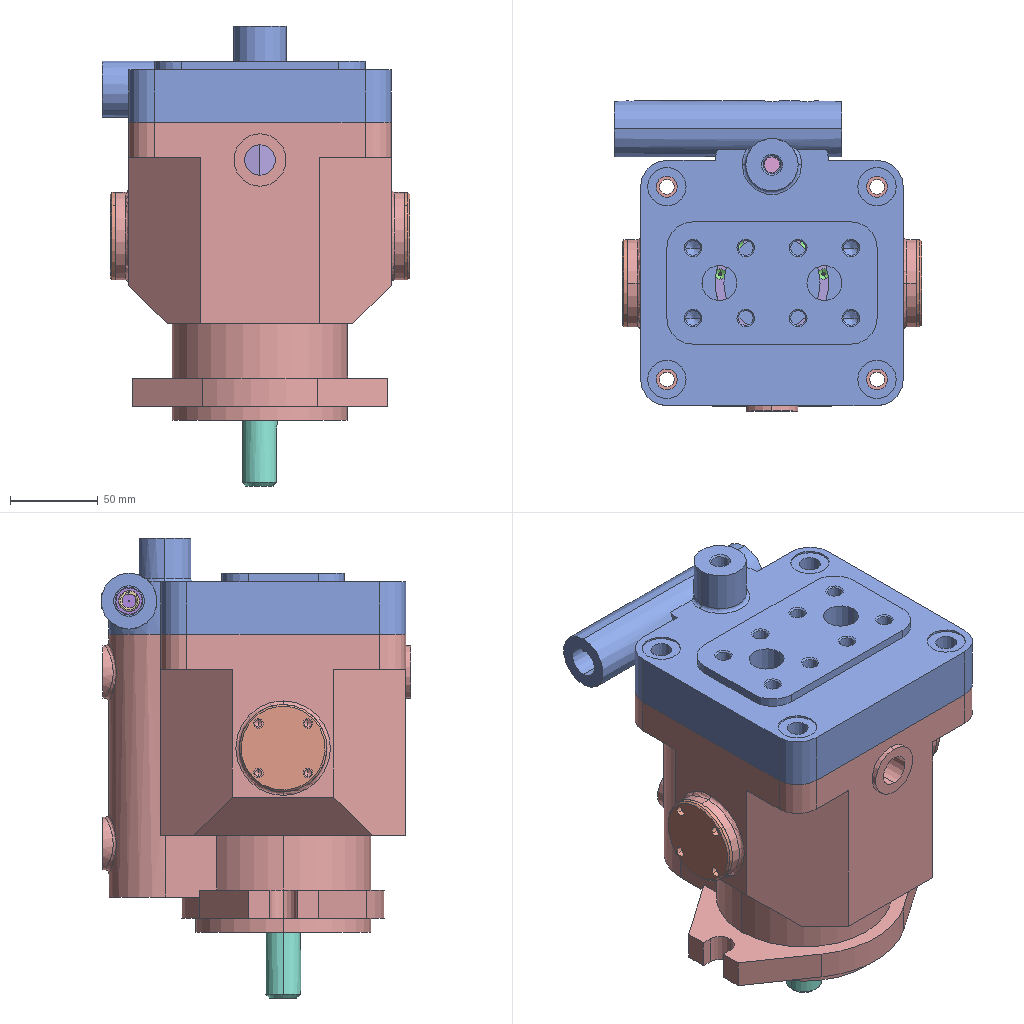Assembly | SolidWorks | 20 different items | 39 placed | box 176 x 177 x 263 mm
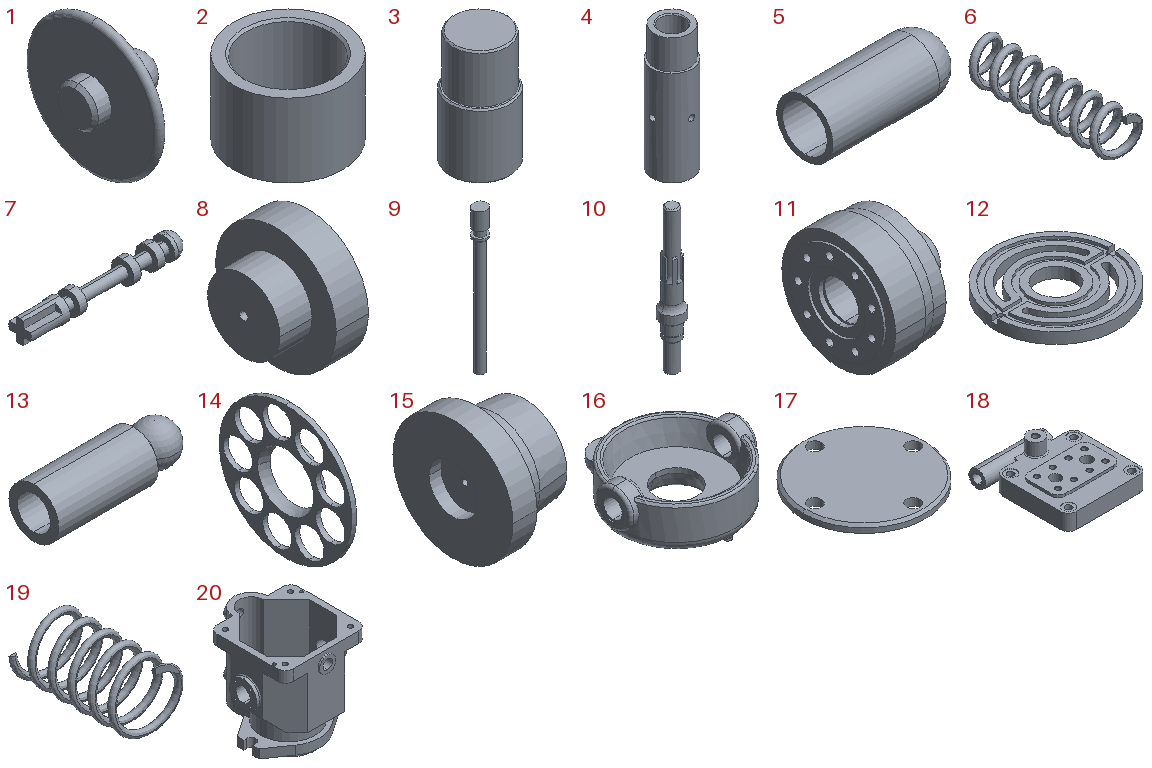Parts list (item | quantity | size | volume | features):
1 | x1 | 22.5 x 40 x 40 mm | 7773 mm3 | features Chamfer 1, Revolution 1
2 | x2 | 26 x 26 x 17.5 mm | 3778 mm3 | features Chamfer 1, Extrusion 1
3 | x2 | 20 x 20 x 37.5 mm | 10804 mm3 | features Chamfer 1, Extrusion 1, ICE 1
4 | x1 | 20 x 20 x 63 mm | 11653 mm3 | features ICE 2, Chamfer 1, CirPattern 1, Extrusion 1, RevCut 1
5 | x1 | 60 x 25 x 25 mm | 11560 mm3 | features ICE 2, Fillet 1, Revolution 1
6 | x1 | 12 x 45 x 12 mm | 746.282 mm3 | features Helix 2, ICE 2, Sweep 2
7 | x1 | 42.5 x 6 x 6 mm | 632.683 mm3 | features ICE 1, Revolution 1
8 | x1 | 8 x 15 x 15 mm | 928.864 mm3 | features Revolution 1
9 | x1 | 9 x 9 x 96 mm | 3208 mm3 | features ICE 2, Chamfer 1, Extrusion 1
10 | x1 | 35 x 35 x 226 mm | 95658 mm3 | features ICE 6, Chamfer 2, CirPattern 1, Extrusion 1, Fillet 1, RevCut 1, RevolvRefSurf 1
11 | x1 | 68 x 90 x 90 mm | 185813 mm3 | features Chamfer 1, CirPattern 1, HoleWzd 1, ICE 1, RevCut 1, Revolution 1
12 | x1 | 90 x 90 x 8 mm | 35911 mm3 | features ICE 4, Extrusion 1
13 | x9 | 42.479 x 15 x 15 mm | 4208 mm3 | features RevCut 1, Revolution 1
14 | x1 | 6 x 82 x 82 mm | 7292 mm3 | features ICE 1, RevCut 1, Revolution 1
15 | x9 | 12 x 20 x 20 mm | 1878 mm3 | features ICE 3, RevCut 1, Revolution 1
16 | x1 | 124 x 138 x 49.724 mm | 237420 mm3 | features ICE 6, Fillet 5, Extrusion 1, HoleWzd 1, MirrorPattern 1, RevCut 1, Sculpt 1, Sweep 1
17 | x2 | 50 x 50 x 3 mm | 5528 mm3 | features Chamfer 1, Extrusion 1, ICE 1
18 | x1 | 165 x 174 x 55 mm | 674925 mm3 | features ICE 17, HoleWzd 8, DelFace 3, 3DProfileFeature 2, SweepCut 2, CombineBodies 1, Extrusion 1, Fillet 1, Revolution 1, Split 1
19 | x1 | 25 x 46 x 25 mm | 1991 mm3 | features Helix 2, ICE 2, Sweep 2
20 | x1 | 165 x 176 x 170 mm | 1139291 mm3 | features ICE 9, HoleWzd 5, Fillet 4, RevCut 2, Revolution 2, Split 2, Chamfer 1, CombineBodies 1, Extrusion 1, MirrorPattern 1
Mates (type | each side: item.copy, entity, surface, feature):
Concentric | 20.1 face cylinder M10 Tapped Hole1 | 18.1 face cylinder Hole1 | 2 times
Concentric | 18.1 face cylinder Cut-Extrude25 | 7.1 face cylinder Revolve1
Concentric | 18.1 face cylinder M12 Tapped Hole3 | assembly face
Concentric | 18.1 face cylinder Cut-Extrude14 | 9.1 face cylinder Boss-Extrude1
Concentric | 18.1 face cylinder Ø5.0mm Dowel Pin Hole 1 | assembly face
Concentric | 20.1 face cylinder Cut-Revolve1 | 10.1 face cylinder Boss-Extrude1
Concentric | 18.1 face cylinder Cut-Extrude6 | 12.1 face cylinder Boss-Extrude1
Coincident | assembly face | 12.1 face plane Cut-Extrude3
Tangent | assembly face | 12.1 face plane Cut-Extrude3
Coincident | 18.1 face plane Boss-Extrude1 | 12.1 face plane Boss-Extrude1
Concentric | 10.1 face cylinder Boss-Extrude5 | 11.1 face cylinder Cut-Revolve1
Coincident | 10.1 face plane Cut-Extrude1 | 11.1 face plane CirPattern1
Parallel | 11.1 plane | assembly plane
Concentric | 11.1 face cylinder Hole1 | 13.1 face cylinder Revolve1
Concentric | 4.1 face cylinder Boss-Extrude2 | 5.1 face cylinder Revolve1
Concentric | 9.1 face cylinder Boss-Extrude1 | 4.1 face cylinder Boss-Extrude2
Coincident | 18.1 face plane Cut-Extrude15 | 4.1 face plane Boss-Extrude1
Coincident | assembly face | 9.1 face plane Boss-Extrude1
Coincident | 9.1 face plane Boss-Extrude1 | 5.1 face plane Cut-Extrude2
Coincident | 4.1 face plane Boss-Extrude1 | 5.1 edge
Coincident | 20.1 face plane Boss-Extrude1 | 18.1 face plane Boss-Extrude1
Tangent | 16.1 face plane Cut-Extrude1 | 5.1 face sphere Revolve1
Concentric | 14.1 face cylinder Revolve1 | 16.1 edge
Parallel | 16.1 plane | assembly plane
Concentric | 14.1 face cylinder Cut-Extrude1 | 15.1 face cylinder Revolve1
Coincident | 14.1 face plane Revolve1 | 15.1 face plane Revolve1
Coincident | 16.1 face plane Cut-Revolve1 | 15.2 face plane Revolve1
Tangent | 13.1 face sphere Revolve1 | 15.2 face sphere Cut-Revolve1
Coincident | 16.1 plane | assembly plane
Concentric | 20.1 face cylinder Cut-Revolve1 | assembly face | 2 times
Coincident | 20.1 face plane Cut-Revolve1 | assembly face | 2 times
Concentric | 10.1 face cylinder Cut-Revolve1 | assembly face
Coincident | 10.1 face plane Cut-Revolve1 | assembly face
Concentric | 20.1 face cylinder Cut-Extrude3 | 17.1 face cylinder Boss-Extrude1
Coincident | 20.1 face plane Boss-Extrude5 | 17.1 face plane Boss-Extrude1
Concentric | 18.1 face cylinder Hole1 | assembly face
Coincident | 18.1 face plane Hole1 | assembly face
Concentric | 20.1 edge | 19.1 select_type:24
Coincident | 20.1 face plane Cut-Extrude2 | 19.1 face plane End Ground
Concentric | 20.1 face cylinder Cut-Extrude2 | 1.1 face cylinder Revolve1
Coincident | 19.1 face plane End Ground | 1.1 face plane Revolve1
Tangent | 16.1 face cone CSK for M6 Hexagon lobular socket raised CTSK head screws1 | 1.1 face sphere Revolve1
Concentric | 20.1 face cylinder Cut-Extrude3 | 2.1 face cylinder Boss-Extrude1
Coincident | 17.1 face plane Boss-Extrude1 | 2.1 face plane Boss-Extrude1
Concentric | 20.1 face cylinder Cut-Extrude3 | 2.2 face cylinder Boss-Extrude1
Coincident | 17.2 face plane Boss-Extrude1 | 2.2 face plane Boss-Extrude1
Concentric | 2.2 face cylinder Boss-Extrude1 | 3.1 face cylinder Boss-Extrude1
Coincident | 17.2 face plane Boss-Extrude1 | 3.1 face plane Boss-Extrude1
Concentric | 2.1 face cylinder Boss-Extrude1 | 3.2 face cylinder Boss-Extrude2
Coincident | 17.1 face plane Boss-Extrude1 | 3.2 face plane Boss-Extrude1
Concentric | 18.1 face cylinder M20 Tapped Hole1 | assembly face
Concentric | 18.1 face cylinder M20 Tapped Hole1 | 8.1 face cylinder Revolve1
Coincident | 18.1 face plane Cut-Extrude24 | 8.1 face plane Revolve1
Concentric | 18.1 face cylinder M20 Tapped Hole1 | 6.1 select_type:24
Coincident | 6.1 face plane End Ground | 8.1 face plane Revolve1
Coincident | assembly face | 6.1 face plane End Ground